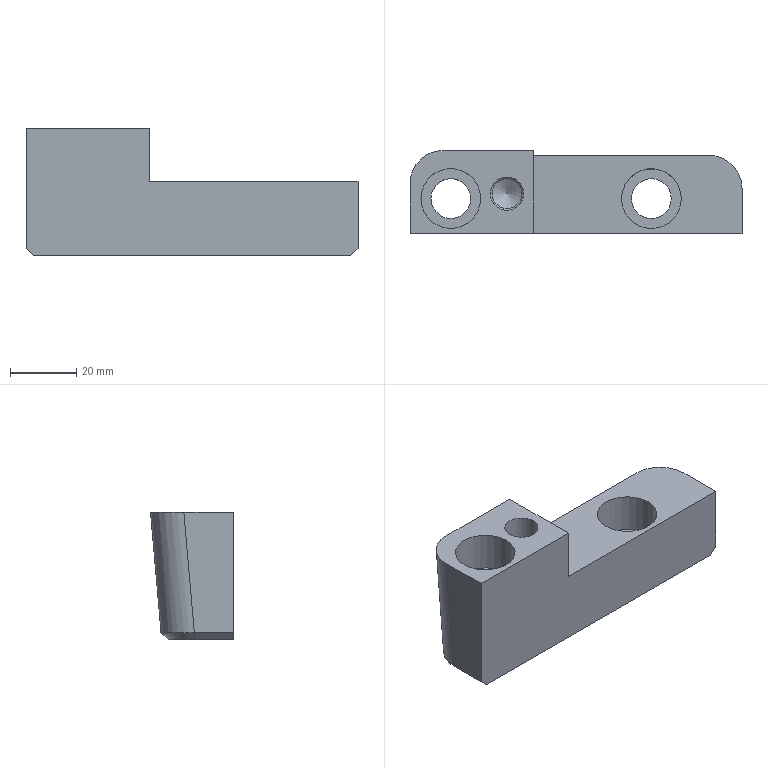Part | STEP file | solid 79 | 1 solid | 25 faces | box 100 x 25 x 38.403 mm | volume 51542 mm3 | plane 13 | cylinder 8 | spline 2 | cone 2 | commonest cylinder face diameters 12 x2 18 x2 20 x2 9 x1 10 x1